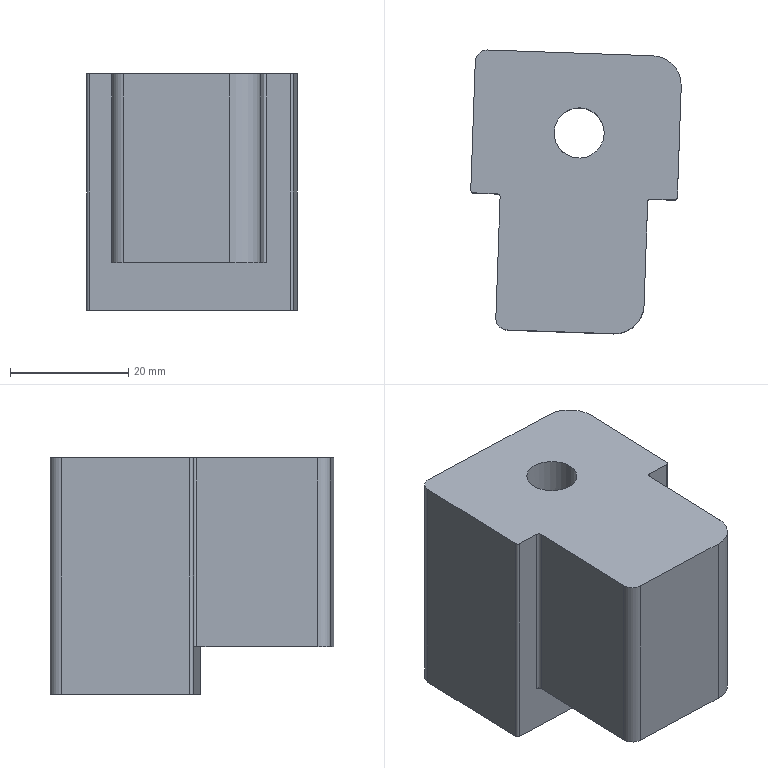Part | NX | features PS-31 2 | 1 solid | 21 faces | box 35.637 x 48.041 x 40 mm | volume 47588 mm3 | plane 11 | cylinder 10 | commonest cylinder face diameters 1 x4 4 x2 10 x2 8.506 x1 14.5 x1
STEP:
#1=CARTESIAN_POINT('',(3392.007,-915.631,900.716));
#2=VERTEX_POINT('',#1);
#3=CARTESIAN_POINT('',(3392.722,-895.143,900.716));
#4=VERTEX_POINT('',#3);
#5=CARTESIAN_POINT('',(3390.831,-949.294,900.716));
#6=DIRECTION('',(-0.0349,-0.9994,0.));
#7=VECTOR('',#6,1000.);
#8=LINE('',#5,#7);
#9=EDGE_CURVE('',#2,#4,#8,.F.);
#10=ORIENTED_EDGE('',*,*,#9,.T.);
#11=CARTESIAN_POINT('',(3392.722,-895.143,868.716));
#12=VERTEX_POINT('',#11);
#13=CARTESIAN_POINT('',(3392.722,-895.143,868.716));
#14=DIRECTION('',(0.,0.,-1.));
#15=VECTOR('',#14,1000.);
#16=LINE('',#13,#15);
#17=EDGE_CURVE('',#4,#12,#16,.T.);
#18=ORIENTED_EDGE('',*,*,#17,.T.);
#19=CARTESIAN_POINT('',(3392.007,-915.631,868.716));
#20=VERTEX_POINT('',#19);
#21=CARTESIAN_POINT('',(3392.334,-906.255,868.716));
#22=DIRECTION('',(0.0349,0.9994,0.));
#23=VECTOR('',#22,1000.);
#24=LINE('',#21,#23);
#25=EDGE_CURVE('',#20,#12,#24,.T.);
#26=ORIENTED_EDGE('',*,*,#25,.F.);
#27=CARTESIAN_POINT('',(3392.007,-915.631,890.716));
#28=DIRECTION('',(0.,0.,1.));
#29=VECTOR('',#28,1000.);
#30=LINE('',#27,#29);
#31=EDGE_CURVE('',#2,#20,#30,.F.);
#32=ORIENTED_EDGE('',*,*,#31,.F.);
#33=EDGE_LOOP('',(#10,#18,#26,#32));
#34=FACE_BOUND('',#33,.T.);
#35=CARTESIAN_POINT('',(3392.52,-900.918,890.716));
#36=DIRECTION('',(0.9994,-0.0349,0.));
#37=DIRECTION('',(-0.0349,-0.9994,0.));
#38=AXIS2_PLACEMENT_3D('',#35,#36,#37);
#39=PLANE('',#38);
#40=ADVANCED_FACE('',(#34),#39,.F.);
#41=CARTESIAN_POINT('',(3393.936,-917.699,900.716));
#42=VERTEX_POINT('',#41);
#43=CARTESIAN_POINT('',(3394.005,-915.701,900.716));
#44=DIRECTION('',(0.,0.,-1.));
#45=DIRECTION('',(0.,1.,0.));
#46=AXIS2_PLACEMENT_3D('',#43,#44,#45);
#47=CIRCLE('',#46,2.);
#48=EDGE_CURVE('',#42,#2,#47,.T.);
#49=ORIENTED_EDGE('',*,*,#48,.T.);
#50=ORIENTED_EDGE('',*,*,#31,.T.);
#51=CARTESIAN_POINT('',(3393.936,-917.699,868.716));
#52=VERTEX_POINT('',#51);
#53=CARTESIAN_POINT('',(3394.005,-915.701,868.716));
#54=DIRECTION('',(0.,0.,-1.));
#55=DIRECTION('',(-1.,0.,0.));
#56=AXIS2_PLACEMENT_3D('',#53,#54,#55);
#57=CIRCLE('',#56,2.);
#58=EDGE_CURVE('',#20,#52,#57,.F.);
#59=ORIENTED_EDGE('',*,*,#58,.T.);
#60=CARTESIAN_POINT('',(3393.936,-917.699,884.716));
#61=DIRECTION('',(0.,0.,1.));
#62=VECTOR('',#61,1000.);
#63=LINE('',#60,#62);
#64=EDGE_CURVE('',#42,#52,#63,.F.);
#65=ORIENTED_EDGE('',*,*,#64,.F.);
#66=EDGE_LOOP('',(#49,#50,#59,#65));
#67=FACE_BOUND('',#66,.T.);
#68=CARTESIAN_POINT('',(3394.005,-915.701,890.716));
#69=DIRECTION('',(0.,0.,1.));
#70=DIRECTION('',(1.,0.,0.));
#71=AXIS2_PLACEMENT_3D('',#68,#69,#70);
#72=CYLINDRICAL_SURFACE('',#71,2.);
#73=ADVANCED_FACE('',(#67),#72,.T.);
#74=CARTESIAN_POINT('',(3411.925,-918.328,868.716));
#75=VERTEX_POINT('',#74);
#76=CARTESIAN_POINT('',(3401.742,-917.972,868.716));
#77=DIRECTION('',(0.9994,-0.0349,0.));
#78=VECTOR('',#77,1000.);
#79=LINE('',#76,#78);
#80=EDGE_CURVE('',#75,#52,#79,.F.);
#81=ORIENTED_EDGE('',*,*,#80,.F.);
#82=CARTESIAN_POINT('',(3411.925,-918.328,900.716));
#83=VERTEX_POINT('',#82);
#84=CARTESIAN_POINT('',(3411.925,-918.328,884.716));
#85=DIRECTION('',(0.,0.,-1.));
#86=VECTOR('',#85,1000.);
#87=LINE('',#84,#86);
#88=EDGE_CURVE('',#83,#75,#87,.T.);
#89=ORIENTED_EDGE('',*,*,#88,.F.);
#90=CARTESIAN_POINT('',(3401.742,-917.972,900.716));
#91=DIRECTION('',(-0.9994,0.0349,0.));
#92=VECTOR('',#91,1000.);
#93=LINE('',#90,#92);
#94=EDGE_CURVE('',#83,#42,#93,.T.);
#95=ORIENTED_EDGE('',*,*,#94,.T.);
#96=ORIENTED_EDGE('',*,*,#64,.T.);
#97=EDGE_LOOP('',(#81,#89,#95,#96));
#98=FACE_BOUND('',#97,.T.);
#99=CARTESIAN_POINT('',(3401.742,-917.972,863.216));
#100=DIRECTION('',(0.0349,0.9994,0.));
#101=DIRECTION('',(-0.9994,0.0349,0.));
#102=AXIS2_PLACEMENT_3D('',#99,#100,#101);
#103=PLANE('',#102);
#104=ADVANCED_FACE('',(#98),#103,.F.);
#105=CARTESIAN_POINT('',(3417.096,-913.505,868.716));
#106=VERTEX_POINT('',#105);
#107=CARTESIAN_POINT('',(3412.099,-913.331,868.716));
#108=DIRECTION('',(0.,0.,-1.));
#109=DIRECTION('',(-1.,0.,0.));
#110=AXIS2_PLACEMENT_3D('',#107,#108,#109);
#111=CIRCLE('',#110,5.);
#112=EDGE_CURVE('',#75,#106,#111,.F.);
#113=ORIENTED_EDGE('',*,*,#112,.T.);
#114=CARTESIAN_POINT('',(3417.096,-913.505,900.716));
#115=VERTEX_POINT('',#114);
#116=CARTESIAN_POINT('',(3417.096,-913.505,935.716));
#117=DIRECTION('',(0.,0.,1.));
#118=VECTOR('',#117,1000.);
#119=LINE('',#116,#118);
#120=EDGE_CURVE('',#106,#115,#119,.T.);
#121=ORIENTED_EDGE('',*,*,#120,.T.);
#122=CARTESIAN_POINT('',(3412.099,-913.331,900.716));
#123=DIRECTION('',(0.,0.,-1.));
#124=DIRECTION('',(0.,1.,0.));
#125=AXIS2_PLACEMENT_3D('',#122,#123,#124);
#126=CIRCLE('',#125,5.);
#127=EDGE_CURVE('',#115,#83,#126,.T.);
#128=ORIENTED_EDGE('',*,*,#127,.T.);
#129=ORIENTED_EDGE('',*,*,#88,.T.);
#130=EDGE_LOOP('',(#113,#121,#128,#129));
#131=FACE_BOUND('',#130,.T.);
#132=CARTESIAN_POINT('',(3412.099,-913.331,935.716));
#133=DIRECTION('',(0.,0.,-1.));
#134=DIRECTION('',(-1.,0.,0.));
#135=AXIS2_PLACEMENT_3D('',#132,#133,#134);
#136=CYLINDRICAL_SURFACE('',#135,5.);
#137=ADVANCED_FACE('',(#131),#136,.T.);
#138=CARTESIAN_POINT('',(3417.707,-896.016,868.716));
#139=VERTEX_POINT('',#138);
#140=CARTESIAN_POINT('',(3417.319,-907.128,868.716));
#141=DIRECTION('',(0.0349,0.9994,0.));
#142=VECTOR('',#141,1000.);
#143=LINE('',#140,#142);
#144=EDGE_CURVE('',#106,#139,#143,.T.);
#145=ORIENTED_EDGE('',*,*,#144,.T.);
#146=CARTESIAN_POINT('',(3417.707,-896.016,900.716));
#147=VERTEX_POINT('',#146);
#148=CARTESIAN_POINT('',(3417.707,-896.016,862.716));
#149=DIRECTION('',(0.,0.,-1.));
#150=VECTOR('',#149,1000.);
#151=LINE('',#148,#150);
#152=EDGE_CURVE('',#139,#147,#151,.F.);
#153=ORIENTED_EDGE('',*,*,#152,.T.);
#154=CARTESIAN_POINT('',(3415.816,-950.166,900.716));
#155=DIRECTION('',(-0.0349,-0.9994,0.));
#156=VECTOR('',#155,1000.);
#157=LINE('',#154,#156);
#158=EDGE_CURVE('',#115,#147,#157,.F.);
#159=ORIENTED_EDGE('',*,*,#158,.F.);
#160=ORIENTED_EDGE('',*,*,#120,.F.);
#161=EDGE_LOOP('',(#145,#153,#159,#160));
#162=FACE_BOUND('',#161,.T.);
#163=CARTESIAN_POINT('',(3417.54,-900.791,862.716));
#164=DIRECTION('',(0.9994,-0.0349,0.));
#165=DIRECTION('',(-0.0349,-0.9994,0.));
#166=AXIS2_PLACEMENT_3D('',#163,#164,#165);
#167=PLANE('',#166);
#168=ADVANCED_FACE('',(#162),#167,.T.);
#169=CARTESIAN_POINT('',(3392.24,-894.626,868.716));
#170=VERTEX_POINT('',#169);
#171=CARTESIAN_POINT('',(3418.224,-895.534,868.716));
#172=VERTEX_POINT('',#171);
#173=CARTESIAN_POINT('',(3405.671,-895.095,868.716));
#174=DIRECTION('',(0.9994,-0.0349,0.));
#175=VECTOR('',#174,1000.);
#176=LINE('',#173,#175);
#177=EDGE_CURVE('',#170,#172,#176,.T.);
#178=ORIENTED_EDGE('',*,*,#177,.T.);
#179=CARTESIAN_POINT('',(3418.206,-896.033,868.716));
#180=DIRECTION('',(0.,0.,-1.));
#181=DIRECTION('',(-1.,0.,0.));
#182=AXIS2_PLACEMENT_3D('',#179,#180,#181);
#183=CIRCLE('',#182,0.5);
#184=EDGE_CURVE('',#172,#139,#183,.F.);
#185=ORIENTED_EDGE('',*,*,#184,.T.);
#186=ORIENTED_EDGE('',*,*,#144,.F.);
#187=ORIENTED_EDGE('',*,*,#112,.F.);
#188=ORIENTED_EDGE('',*,*,#80,.T.);
#189=ORIENTED_EDGE('',*,*,#58,.F.);
#190=ORIENTED_EDGE('',*,*,#25,.T.);
#191=CARTESIAN_POINT('',(3392.222,-895.126,868.716));
#192=DIRECTION('',(0.,0.,-1.));
#193=DIRECTION('',(-1.,0.,0.));
#194=AXIS2_PLACEMENT_3D('',#191,#192,#193);
#195=CIRCLE('',#194,0.5);
#196=EDGE_CURVE('',#12,#170,#195,.F.);
#197=ORIENTED_EDGE('',*,*,#196,.T.);
#198=EDGE_LOOP('',(#178,#185,#186,#187,#188,#189,#190,#197));
#199=FACE_BOUND('',#198,.T.);
#200=CARTESIAN_POINT('',(3405.266,-906.707,868.716));
#201=DIRECTION('',(0.,0.,-1.));
#202=DIRECTION('',(-0.0349,-0.9994,0.));
#203=AXIS2_PLACEMENT_3D('',#200,#201,#202);
#204=PLANE('',#203);
#205=ADVANCED_FACE('',(#199),#204,.T.);
#206=CARTESIAN_POINT('',(3392.24,-894.626,900.716));
#207=VERTEX_POINT('',#206);
#208=CARTESIAN_POINT('',(3392.222,-895.126,900.716));
#209=DIRECTION('',(0.,0.,-1.));
#210=DIRECTION('',(0.,1.,0.));
#211=AXIS2_PLACEMENT_3D('',#208,#209,#210);
#212=CIRCLE('',#211,0.5);
#213=EDGE_CURVE('',#207,#4,#212,.T.);
#214=ORIENTED_EDGE('',*,*,#213,.T.);
#215=ORIENTED_EDGE('',*,*,#9,.F.);
#216=ORIENTED_EDGE('',*,*,#48,.F.);
#217=ORIENTED_EDGE('',*,*,#94,.F.);
#218=ORIENTED_EDGE('',*,*,#127,.F.);
#219=ORIENTED_EDGE('',*,*,#158,.T.);
#220=CARTESIAN_POINT('',(3418.224,-895.534,900.716));
#221=VERTEX_POINT('',#220);
#222=CARTESIAN_POINT('',(3418.206,-896.033,900.716));
#223=DIRECTION('',(0.,0.,-1.));
#224=DIRECTION('',(0.,1.,0.));
#225=AXIS2_PLACEMENT_3D('',#222,#223,#224);
#226=CIRCLE('',#225,0.5);
#227=EDGE_CURVE('',#147,#221,#226,.T.);
#228=ORIENTED_EDGE('',*,*,#227,.T.);
#229=CARTESIAN_POINT('',(3422.221,-895.673,900.716));
#230=VERTEX_POINT('',#229);
#231=CARTESIAN_POINT('',(3402.542,-894.986,900.716));
#232=DIRECTION('',(-0.9994,0.0349,0.));
#233=VECTOR('',#232,1000.);
#234=LINE('',#231,#233);
#235=EDGE_CURVE('',#221,#230,#234,.F.);
#236=ORIENTED_EDGE('',*,*,#235,.T.);
#237=CARTESIAN_POINT('',(3422.739,-895.191,900.716));
#238=VERTEX_POINT('',#237);
#239=CARTESIAN_POINT('',(3422.239,-895.173,900.716));
#240=DIRECTION('',(0.,0.,-1.));
#241=DIRECTION('',(0.,1.,0.));
#242=AXIS2_PLACEMENT_3D('',#239,#240,#241);
#243=CIRCLE('',#242,0.5);
#244=EDGE_CURVE('',#230,#238,#243,.F.);
#245=ORIENTED_EDGE('',*,*,#244,.T.);
#246=CARTESIAN_POINT('',(3423.393,-876.439,900.716));
#247=VERTEX_POINT('',#246);
#248=CARTESIAN_POINT('',(3420.813,-950.34,900.716));
#249=DIRECTION('',(-0.0349,-0.9994,0.));
#250=VECTOR('',#249,1000.);
#251=LINE('',#248,#250);
#252=EDGE_CURVE('',#238,#247,#251,.F.);
#253=ORIENTED_EDGE('',*,*,#252,.T.);
#254=CARTESIAN_POINT('',(3418.571,-871.268,900.716));
#255=VERTEX_POINT('',#254);
#256=CARTESIAN_POINT('',(3418.396,-876.265,900.716));
#257=DIRECTION('',(0.,0.,-1.));
#258=DIRECTION('',(0.,1.,0.));
#259=AXIS2_PLACEMENT_3D('',#256,#257,#258);
#260=CIRCLE('',#259,5.);
#261=EDGE_CURVE('',#255,#247,#260,.T.);
#262=ORIENTED_EDGE('',*,*,#261,.F.);
#263=CARTESIAN_POINT('',(3390.588,-870.291,900.716));
#264=VERTEX_POINT('',#263);
#265=CARTESIAN_POINT('',(3247.679,-865.301,900.716));
#266=DIRECTION('',(-0.9994,0.0349,0.));
#267=VECTOR('',#266,1000.);
#268=LINE('',#265,#267);
#269=EDGE_CURVE('',#255,#264,#268,.T.);
#270=ORIENTED_EDGE('',*,*,#269,.T.);
#271=CARTESIAN_POINT('',(3388.519,-872.22,900.716));
#272=VERTEX_POINT('',#271);
#273=CARTESIAN_POINT('',(3390.518,-872.29,900.716));
#274=DIRECTION('',(0.,0.,-1.));
#275=DIRECTION('',(0.,1.,0.));
#276=AXIS2_PLACEMENT_3D('',#273,#274,#275);
#277=CIRCLE('',#276,2.);
#278=EDGE_CURVE('',#272,#264,#277,.T.);
#279=ORIENTED_EDGE('',*,*,#278,.F.);
#280=CARTESIAN_POINT('',(3387.76,-893.97,900.716));
#281=VERTEX_POINT('',#280);
#282=CARTESIAN_POINT('',(3385.834,-949.119,900.716));
#283=DIRECTION('',(-0.0349,-0.9994,0.));
#284=VECTOR('',#283,1000.);
#285=LINE('',#282,#284);
#286=EDGE_CURVE('',#281,#272,#285,.F.);
#287=ORIENTED_EDGE('',*,*,#286,.F.);
#288=CARTESIAN_POINT('',(3388.242,-894.487,900.716));
#289=VERTEX_POINT('',#288);
#290=CARTESIAN_POINT('',(3388.26,-893.987,900.716));
#291=DIRECTION('',(0.,0.,-1.));
#292=DIRECTION('',(0.,1.,0.));
#293=AXIS2_PLACEMENT_3D('',#290,#291,#292);
#294=CIRCLE('',#293,0.5);
#295=EDGE_CURVE('',#281,#289,#294,.F.);
#296=ORIENTED_EDGE('',*,*,#295,.T.);
#297=CARTESIAN_POINT('',(3402.542,-894.986,900.716));
#298=DIRECTION('',(-0.9994,0.0349,0.));
#299=VECTOR('',#298,1000.);
#300=LINE('',#297,#299);
#301=EDGE_CURVE('',#289,#207,#300,.F.);
#302=ORIENTED_EDGE('',*,*,#301,.T.);
#303=EDGE_LOOP('',(#214,#215,#216,#217,#218,#219,#228,#236,#245,#253,#262,#270,#279,#287,#296,#302));
#304=FACE_BOUND('',#303,.T.);
#305=CARTESIAN_POINT('',(3406.107,-880.088,900.716));
#306=VERTEX_POINT('',#305);
#307=CARTESIAN_POINT('',(3406.107,-884.341,900.716));
#308=DIRECTION('',(0.,0.,-1.));
#309=DIRECTION('',(0.,1.,0.));
#310=AXIS2_PLACEMENT_3D('',#307,#308,#309);
#311=CIRCLE('',#310,4.253);
#312=EDGE_CURVE('',#306,#306,#311,.F.);
#313=ORIENTED_EDGE('',*,*,#312,.F.);
#314=EDGE_LOOP('',(#313));
#315=FACE_BOUND('',#314,.T.);
#316=CARTESIAN_POINT('',(3244.924,-944.199,900.716));
#317=DIRECTION('',(0.,0.,1.));
#318=DIRECTION('',(0.9976,-0.06975,0.));
#319=AXIS2_PLACEMENT_3D('',#316,#317,#318);
#320=PLANE('',#319);
#321=ADVANCED_FACE('',(#304,#315),#320,.T.);
#322=ORIENTED_EDGE('',*,*,#213,.F.);
#323=CARTESIAN_POINT('',(3392.24,-894.626,890.716));
#324=DIRECTION('',(0.,0.,-1.));
#325=VECTOR('',#324,1000.);
#326=LINE('',#323,#325);
#327=EDGE_CURVE('',#170,#207,#326,.F.);
#328=ORIENTED_EDGE('',*,*,#327,.F.);
#329=ORIENTED_EDGE('',*,*,#196,.F.);
#330=ORIENTED_EDGE('',*,*,#17,.F.);
#331=EDGE_LOOP('',(#322,#328,#329,#330));
#332=FACE_BOUND('',#331,.T.);
#333=CARTESIAN_POINT('',(3392.222,-895.126,890.716));
#334=DIRECTION('',(0.,0.,1.));
#335=DIRECTION('',(1.,0.,0.));
#336=AXIS2_PLACEMENT_3D('',#333,#334,#335);
#337=CYLINDRICAL_SURFACE('',#336,0.5);
#338=ADVANCED_FACE('',(#332),#337,.F.);
#339=ORIENTED_EDGE('',*,*,#227,.F.);
#340=ORIENTED_EDGE('',*,*,#152,.F.);
#341=ORIENTED_EDGE('',*,*,#184,.F.);
#342=CARTESIAN_POINT('',(3418.224,-895.534,863.216));
#343=DIRECTION('',(0.,0.,-1.));
#344=VECTOR('',#343,1000.);
#345=LINE('',#342,#344);
#346=EDGE_CURVE('',#221,#172,#345,.T.);
#347=ORIENTED_EDGE('',*,*,#346,.F.);
#348=EDGE_LOOP('',(#339,#340,#341,#347));
#349=FACE_BOUND('',#348,.T.);
#350=CARTESIAN_POINT('',(3418.206,-896.033,863.216));
#351=DIRECTION('',(0.,0.,-1.));
#352=DIRECTION('',(-1.,0.,0.));
#353=AXIS2_PLACEMENT_3D('',#350,#351,#352);
#354=CYLINDRICAL_SURFACE('',#353,0.5);
#355=ADVANCED_FACE('',(#349),#354,.F.);
#356=ORIENTED_EDGE('',*,*,#301,.F.);
#357=CARTESIAN_POINT('',(3388.242,-894.487,860.716));
#358=VERTEX_POINT('',#357);
#359=CARTESIAN_POINT('',(3388.242,-894.487,863.216));
#360=DIRECTION('',(0.,0.,1.));
#361=VECTOR('',#360,1000.);
#362=LINE('',#359,#361);
#363=EDGE_CURVE('',#289,#358,#362,.F.);
#364=ORIENTED_EDGE('',*,*,#363,.T.);
#365=CARTESIAN_POINT('',(3422.221,-895.673,860.716));
#366=VERTEX_POINT('',#365);
#367=CARTESIAN_POINT('',(2864.539,-876.201,860.716));
#368=DIRECTION('',(0.9994,-0.0349,0.));
#369=VECTOR('',#368,1000.);
#370=LINE('',#367,#369);
#371=EDGE_CURVE('',#366,#358,#370,.F.);
#372=ORIENTED_EDGE('',*,*,#371,.F.);
#373=CARTESIAN_POINT('',(3422.221,-895.673,890.716));
#374=DIRECTION('',(0.,0.,1.));
#375=VECTOR('',#374,1000.);
#376=LINE('',#373,#375);
#377=EDGE_CURVE('',#366,#230,#376,.T.);
#378=ORIENTED_EDGE('',*,*,#377,.T.);
#379=ORIENTED_EDGE('',*,*,#235,.F.);
#380=ORIENTED_EDGE('',*,*,#346,.T.);
#381=ORIENTED_EDGE('',*,*,#177,.F.);
#382=ORIENTED_EDGE('',*,*,#327,.T.);
#383=EDGE_LOOP('',(#356,#364,#372,#378,#379,#380,#381,#382));
#384=FACE_BOUND('',#383,.T.);
#385=CARTESIAN_POINT('',(3402.542,-894.986,863.216));
#386=DIRECTION('',(0.0349,0.9994,0.));
#387=DIRECTION('',(-0.9994,0.0349,0.));
#388=AXIS2_PLACEMENT_3D('',#385,#386,#387);
#389=PLANE('',#388);
#390=ADVANCED_FACE('',(#384),#389,.F.);
#391=CARTESIAN_POINT('',(3413.357,-884.341,860.716));
#392=VERTEX_POINT('',#391);
#393=CARTESIAN_POINT('',(3406.107,-884.341,860.716));
#394=DIRECTION('',(0.,0.,-1.));
#395=DIRECTION('',(1.,0.,0.));
#396=AXIS2_PLACEMENT_3D('',#393,#394,#395);
#397=CIRCLE('',#396,7.25);
#398=EDGE_CURVE('',#392,#392,#397,.T.);
#399=ORIENTED_EDGE('',*,*,#398,.F.);
#400=EDGE_LOOP('',(#399));
#401=FACE_BOUND('',#400,.T.);
#402=CARTESIAN_POINT('',(3387.76,-893.97,860.716));
#403=VERTEX_POINT('',#402);
#404=CARTESIAN_POINT('',(3388.26,-893.987,860.716));
#405=DIRECTION('',(0.,0.,-1.));
#406=DIRECTION('',(1.,0.,0.));
#407=AXIS2_PLACEMENT_3D('',#404,#405,#406);
#408=CIRCLE('',#407,0.5);
#409=EDGE_CURVE('',#358,#403,#408,.T.);
#410=ORIENTED_EDGE('',*,*,#409,.T.);
#411=CARTESIAN_POINT('',(3388.519,-872.22,860.716));
#412=VERTEX_POINT('',#411);
#413=CARTESIAN_POINT('',(3393.297,-735.391,860.716));
#414=DIRECTION('',(-0.0349,-0.9994,0.));
#415=VECTOR('',#414,1000.);
#416=LINE('',#413,#415);
#417=EDGE_CURVE('',#403,#412,#416,.F.);
#418=ORIENTED_EDGE('',*,*,#417,.T.);
#419=CARTESIAN_POINT('',(3390.588,-870.291,860.716));
#420=VERTEX_POINT('',#419);
#421=CARTESIAN_POINT('',(3390.518,-872.29,860.716));
#422=DIRECTION('',(0.,0.,-1.));
#423=DIRECTION('',(1.,0.,0.));
#424=AXIS2_PLACEMENT_3D('',#421,#422,#423);
#425=CIRCLE('',#424,2.);
#426=EDGE_CURVE('',#420,#412,#425,.F.);
#427=ORIENTED_EDGE('',*,*,#426,.F.);
#428=CARTESIAN_POINT('',(3418.571,-871.268,860.716));
#429=VERTEX_POINT('',#428);
#430=CARTESIAN_POINT('',(3377.596,-869.837,860.716));
#431=DIRECTION('',(0.9994,-0.0349,0.));
#432=VECTOR('',#431,1000.);
#433=LINE('',#430,#432);
#434=EDGE_CURVE('',#420,#429,#433,.T.);
#435=ORIENTED_EDGE('',*,*,#434,.T.);
#436=CARTESIAN_POINT('',(3423.393,-876.439,860.716));
#437=VERTEX_POINT('',#436);
#438=CARTESIAN_POINT('',(3418.396,-876.265,860.716));
#439=DIRECTION('',(0.,0.,-1.));
#440=DIRECTION('',(1.,0.,0.));
#441=AXIS2_PLACEMENT_3D('',#438,#439,#440);
#442=CIRCLE('',#441,5.);
#443=EDGE_CURVE('',#437,#429,#442,.F.);
#444=ORIENTED_EDGE('',*,*,#443,.F.);
#445=CARTESIAN_POINT('',(3422.739,-895.191,860.716));
#446=VERTEX_POINT('',#445);
#447=CARTESIAN_POINT('',(3428.276,-736.613,860.716));
#448=DIRECTION('',(-0.0349,-0.9994,0.));
#449=VECTOR('',#448,1000.);
#450=LINE('',#447,#449);
#451=EDGE_CURVE('',#446,#437,#450,.F.);
#452=ORIENTED_EDGE('',*,*,#451,.F.);
#453=CARTESIAN_POINT('',(3422.239,-895.173,860.716));
#454=DIRECTION('',(0.,0.,-1.));
#455=DIRECTION('',(1.,0.,0.));
#456=AXIS2_PLACEMENT_3D('',#453,#454,#455);
#457=CIRCLE('',#456,0.5);
#458=EDGE_CURVE('',#446,#366,#457,.T.);
#459=ORIENTED_EDGE('',*,*,#458,.T.);
#460=ORIENTED_EDGE('',*,*,#371,.T.);
#461=EDGE_LOOP('',(#410,#418,#427,#435,#444,#452,#459,#460));
#462=FACE_BOUND('',#461,.T.);
#463=CARTESIAN_POINT('',(2870.094,-717.123,860.716));
#464=DIRECTION('',(0.,0.,1.));
#465=DIRECTION('',(0.,-1.,0.));
#466=AXIS2_PLACEMENT_3D('',#463,#464,#465);
#467=PLANE('',#466);
#468=ADVANCED_FACE('',(#401,#462),#467,.F.);
#469=ORIENTED_EDGE('',*,*,#252,.F.);
#470=CARTESIAN_POINT('',(3422.739,-895.191,868.716));
#471=DIRECTION('',(0.,0.,1.));
#472=VECTOR('',#471,1000.);
#473=LINE('',#470,#472);
#474=EDGE_CURVE('',#238,#446,#473,.F.);
#475=ORIENTED_EDGE('',*,*,#474,.T.);
#476=ORIENTED_EDGE('',*,*,#451,.T.);
#477=CARTESIAN_POINT('',(3423.393,-876.439,862.716));
#478=DIRECTION('',(0.,0.,1.));
#479=VECTOR('',#478,1000.);
#480=LINE('',#477,#479);
#481=EDGE_CURVE('',#247,#437,#480,.F.);
#482=ORIENTED_EDGE('',*,*,#481,.F.);
#483=EDGE_LOOP('',(#469,#475,#476,#482));
#484=FACE_BOUND('',#483,.T.);
#485=CARTESIAN_POINT('',(3422.537,-900.966,862.716));
#486=DIRECTION('',(0.9994,-0.0349,0.));
#487=DIRECTION('',(-0.0349,-0.9994,0.));
#488=AXIS2_PLACEMENT_3D('',#485,#486,#487);
#489=PLANE('',#488);
#490=ADVANCED_FACE('',(#484),#489,.T.);
#491=ORIENTED_EDGE('',*,*,#434,.F.);
#492=CARTESIAN_POINT('',(3390.588,-870.291,860.716));
#493=DIRECTION('',(0.,0.,-1.));
#494=VECTOR('',#493,1000.);
#495=LINE('',#492,#494);
#496=EDGE_CURVE('',#264,#420,#495,.T.);
#497=ORIENTED_EDGE('',*,*,#496,.F.);
#498=ORIENTED_EDGE('',*,*,#269,.F.);
#499=CARTESIAN_POINT('',(3418.571,-871.268,935.716));
#500=DIRECTION('',(0.,0.,-1.));
#501=VECTOR('',#500,1000.);
#502=LINE('',#499,#501);
#503=EDGE_CURVE('',#429,#255,#502,.F.);
#504=ORIENTED_EDGE('',*,*,#503,.F.);
#505=EDGE_LOOP('',(#491,#497,#498,#504));
#506=FACE_BOUND('',#505,.T.);
#507=CARTESIAN_POINT('',(3377.596,-869.837,935.716));
#508=DIRECTION('',(-0.0349,-0.9994,0.));
#509=DIRECTION('',(-0.9994,0.0349,0.));
#510=AXIS2_PLACEMENT_3D('',#507,#508,#509);
#511=PLANE('',#510);
#512=ADVANCED_FACE('',(#506),#511,.F.);
#513=ORIENTED_EDGE('',*,*,#417,.F.);
#514=CARTESIAN_POINT('',(3387.76,-893.97,890.716));
#515=DIRECTION('',(0.,0.,1.));
#516=VECTOR('',#515,1000.);
#517=LINE('',#514,#516);
#518=EDGE_CURVE('',#403,#281,#517,.T.);
#519=ORIENTED_EDGE('',*,*,#518,.T.);
#520=ORIENTED_EDGE('',*,*,#286,.T.);
#521=CARTESIAN_POINT('',(3388.519,-872.22,890.716));
#522=DIRECTION('',(0.,0.,1.));
#523=VECTOR('',#522,1000.);
#524=LINE('',#521,#523);
#525=EDGE_CURVE('',#412,#272,#524,.T.);
#526=ORIENTED_EDGE('',*,*,#525,.F.);
#527=EDGE_LOOP('',(#513,#519,#520,#526));
#528=FACE_BOUND('',#527,.T.);
#529=CARTESIAN_POINT('',(3387.523,-900.744,890.716));
#530=DIRECTION('',(0.9994,-0.0349,0.));
#531=DIRECTION('',(-0.0349,-0.9994,0.));
#532=AXIS2_PLACEMENT_3D('',#529,#530,#531);
#533=PLANE('',#532);
#534=ADVANCED_FACE('',(#528),#533,.F.);
#535=ORIENTED_EDGE('',*,*,#278,.T.);
#536=ORIENTED_EDGE('',*,*,#496,.T.);
#537=ORIENTED_EDGE('',*,*,#426,.T.);
#538=ORIENTED_EDGE('',*,*,#525,.T.);
#539=EDGE_LOOP('',(#535,#536,#537,#538));
#540=FACE_BOUND('',#539,.T.);
#541=CARTESIAN_POINT('',(3390.518,-872.29,935.716));
#542=DIRECTION('',(0.,0.,-1.));
#543=DIRECTION('',(-0.9976,0.06975,0.));
#544=AXIS2_PLACEMENT_3D('',#541,#542,#543);
#545=CYLINDRICAL_SURFACE('',#544,2.);
#546=ADVANCED_FACE('',(#540),#545,.T.);
#547=ORIENTED_EDGE('',*,*,#261,.T.);
#548=ORIENTED_EDGE('',*,*,#481,.T.);
#549=ORIENTED_EDGE('',*,*,#443,.T.);
#550=ORIENTED_EDGE('',*,*,#503,.T.);
#551=EDGE_LOOP('',(#547,#548,#549,#550));
#552=FACE_BOUND('',#551,.T.);
#553=CARTESIAN_POINT('',(3418.396,-876.265,862.716));
#554=DIRECTION('',(0.,0.,1.));
#555=DIRECTION('',(0.9976,-0.06975,0.));
#556=AXIS2_PLACEMENT_3D('',#553,#554,#555);
#557=CYLINDRICAL_SURFACE('',#556,5.);
#558=ADVANCED_FACE('',(#552),#557,.T.);
#559=CARTESIAN_POINT('',(3410.35,-884.638,879.716));
#560=VERTEX_POINT('',#559);
#561=CARTESIAN_POINT('',(3406.107,-884.341,879.716));
#562=DIRECTION('',(0.,0.,-1.));
#563=DIRECTION('',(0.9976,-0.06975,0.));
#564=AXIS2_PLACEMENT_3D('',#561,#562,#563);
#565=CIRCLE('',#564,4.253);
#566=EDGE_CURVE('',#560,#560,#565,.T.);
#567=ORIENTED_EDGE('',*,*,#566,.T.);
#568=EDGE_LOOP('',(#567));
#569=FACE_BOUND('',#568,.T.);
#570=ORIENTED_EDGE('',*,*,#312,.T.);
#571=EDGE_LOOP('',(#570));
#572=FACE_BOUND('',#571,.T.);
#573=CARTESIAN_POINT('',(3406.107,-884.341,868.716));
#574=DIRECTION('',(0.,0.,1.));
#575=DIRECTION('',(0.9976,-0.06975,0.));
#576=AXIS2_PLACEMENT_3D('',#573,#574,#575);
#577=CYLINDRICAL_SURFACE('',#576,4.253);
#578=ADVANCED_FACE('',(#569,#572),#577,.F.);
#579=ORIENTED_EDGE('',*,*,#566,.F.);
#580=EDGE_LOOP('',(#579));
#581=FACE_BOUND('',#580,.T.);
#582=CARTESIAN_POINT('',(3413.339,-884.847,879.716));
#583=VERTEX_POINT('',#582);
#584=CARTESIAN_POINT('',(3406.107,-884.341,879.716));
#585=DIRECTION('',(0.,0.,1.));
#586=DIRECTION('',(0.9976,-0.06975,0.));
#587=AXIS2_PLACEMENT_3D('',#584,#585,#586);
#588=CIRCLE('',#587,7.25);
#589=EDGE_CURVE('',#583,#583,#588,.F.);
#590=ORIENTED_EDGE('',*,*,#589,.T.);
#591=EDGE_LOOP('',(#590));
#592=FACE_BOUND('',#591,.T.);
#593=CARTESIAN_POINT('',(3406.107,-884.341,879.716));
#594=DIRECTION('',(0.,0.,1.));
#595=DIRECTION('',(0.9976,-0.06975,0.));
#596=AXIS2_PLACEMENT_3D('',#593,#594,#595);
#597=PLANE('',#596);
#598=ADVANCED_FACE('',(#581,#592),#597,.F.);
#599=ORIENTED_EDGE('',*,*,#589,.F.);
#600=EDGE_LOOP('',(#599));
#601=FACE_BOUND('',#600,.T.);
#602=ORIENTED_EDGE('',*,*,#398,.T.);
#603=EDGE_LOOP('',(#602));
#604=FACE_BOUND('',#603,.T.);
#605=CARTESIAN_POINT('',(3406.107,-884.341,868.716));
#606=DIRECTION('',(0.,0.,1.));
#607=DIRECTION('',(0.9976,-0.06975,0.));
#608=AXIS2_PLACEMENT_3D('',#605,#606,#607);
#609=CYLINDRICAL_SURFACE('',#608,7.25);
#610=ADVANCED_FACE('',(#601,#604),#609,.F.);
#611=ORIENTED_EDGE('',*,*,#458,.F.);
#612=ORIENTED_EDGE('',*,*,#474,.F.);
#613=ORIENTED_EDGE('',*,*,#244,.F.);
#614=ORIENTED_EDGE('',*,*,#377,.F.);
#615=EDGE_LOOP('',(#611,#612,#613,#614));
#616=FACE_BOUND('',#615,.T.);
#617=CARTESIAN_POINT('',(3422.239,-895.173,863.216));
#618=DIRECTION('',(0.,0.,-1.));
#619=DIRECTION('',(-1.,0.,0.));
#620=AXIS2_PLACEMENT_3D('',#617,#618,#619);
#621=CYLINDRICAL_SURFACE('',#620,0.5);
#622=ADVANCED_FACE('',(#616),#621,.T.);
#623=ORIENTED_EDGE('',*,*,#409,.F.);
#624=ORIENTED_EDGE('',*,*,#363,.F.);
#625=ORIENTED_EDGE('',*,*,#295,.F.);
#626=ORIENTED_EDGE('',*,*,#518,.F.);
#627=EDGE_LOOP('',(#623,#624,#625,#626));
#628=FACE_BOUND('',#627,.T.);
#629=CARTESIAN_POINT('',(3388.26,-893.987,890.716));
#630=DIRECTION('',(0.,0.,1.));
#631=DIRECTION('',(1.,0.,0.));
#632=AXIS2_PLACEMENT_3D('',#629,#630,#631);
#633=CYLINDRICAL_SURFACE('',#632,0.5);
#634=ADVANCED_FACE('',(#628),#633,.T.);
#635=CLOSED_SHELL('',(#40,#73,#104,#137,#168,#205,#321,#338,#355,#390,#468,#490,#512,#534,#546,#558,#578,#598,#610,#622,#634));
#636=MANIFOLD_SOLID_BREP('',#635);
#637=(LENGTH_UNIT()NAMED_UNIT(*)SI_UNIT(.MILLI.,.METRE.));
#638=UNCERTAINTY_MEASURE_WITH_UNIT(LENGTH_MEASURE(0.00001),#637,'','');
#639=(NAMED_UNIT(*)PLANE_ANGLE_UNIT()SI_UNIT($,.RADIAN.));
#640=(NAMED_UNIT(*)SI_UNIT($,.STERADIAN.)SOLID_ANGLE_UNIT());
#641=(GEOMETRIC_REPRESENTATION_CONTEXT(3)GLOBAL_UNCERTAINTY_ASSIGNED_CONTEXT((#638))GLOBAL_UNIT_ASSIGNED_CONTEXT((#637,#639,#640))REPRESENTATION_CONTEXT('',''));
#642=ADVANCED_BREP_SHAPE_REPRESENTATION('',(#636),#641);